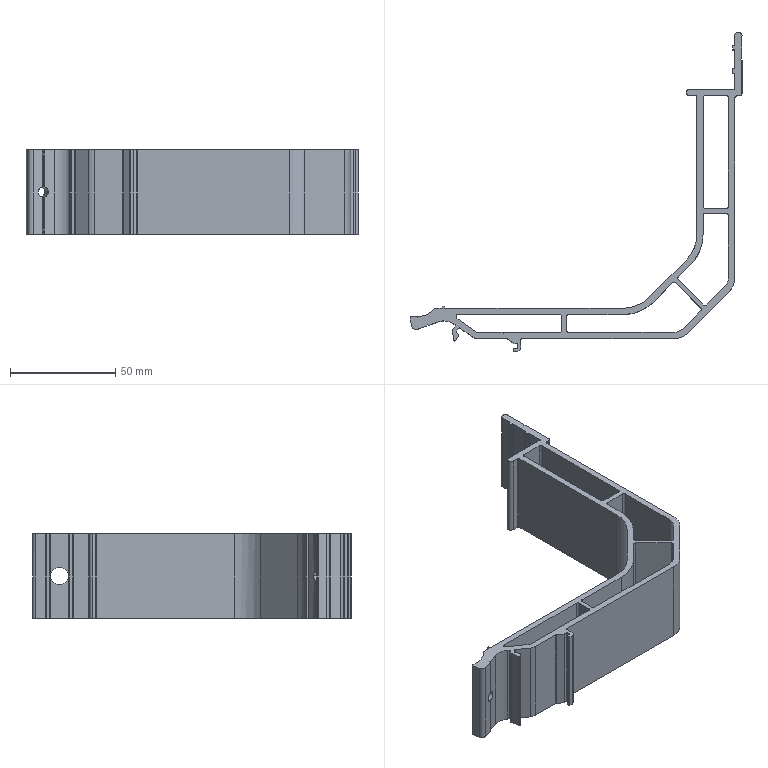Part | STEP file | V00-000000447 | 1 solid | 158 faces | box 157.7 x 151.5 x 40 mm | volume 68710 mm3 | plane 82 | cylinder 76 | commonest cylinder face diameters 0.6 x28 2 x20 3 x5 1 x4 0.4 x2 4 x2